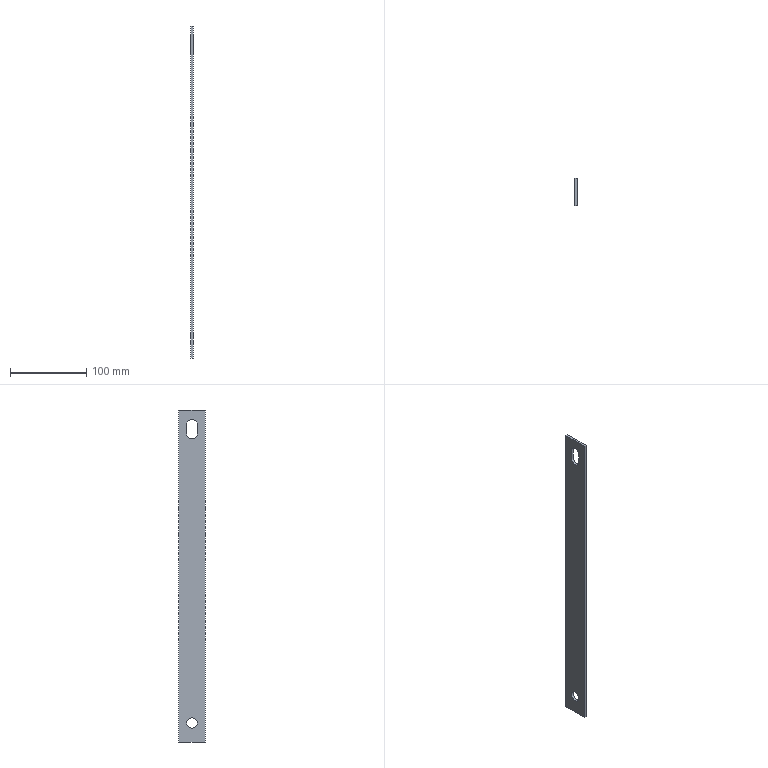Part | NX | features solid 2 | 1 solid | 11 faces | box 3 x 35 x 435 mm | volume 44310 mm3 | plane 8 | cylinder 3 | commonest cylinder face diameters 13.5 x3
STEP:
#1=CARTESIAN_POINT('',(1130.,-198.25,251.25));
#2=VERTEX_POINT('',#1);
#3=CARTESIAN_POINT('',(1130.,-211.75,251.25));
#4=VERTEX_POINT('',#3);
#5=CARTESIAN_POINT('',(1130.,-205.,251.25));
#6=DIRECTION('',(1.,0.,0.));
#7=DIRECTION('',(0.,1.,0.));
#8=AXIS2_PLACEMENT_3D('',#5,#6,#7);
#9=CIRCLE('',#8,6.75);
#10=EDGE_CURVE('',#2,#4,#9,.T.);
#11=ORIENTED_EDGE('',*,*,#10,.F.);
#12=CARTESIAN_POINT('',(1133.,-198.25,251.25));
#13=VERTEX_POINT('',#12);
#14=CARTESIAN_POINT('',(1133.,-198.25,251.25));
#15=DIRECTION('',(-1.,0.,0.));
#16=VECTOR('',#15,1000.);
#17=LINE('',#14,#16);
#18=EDGE_CURVE('',#13,#2,#17,.T.);
#19=ORIENTED_EDGE('',*,*,#18,.F.);
#20=CARTESIAN_POINT('',(1133.,-211.75,251.25));
#21=VERTEX_POINT('',#20);
#22=CARTESIAN_POINT('',(1133.,-205.,251.25));
#23=DIRECTION('',(1.,0.,0.));
#24=DIRECTION('',(0.,1.,0.));
#25=AXIS2_PLACEMENT_3D('',#22,#23,#24);
#26=CIRCLE('',#25,6.75);
#27=EDGE_CURVE('',#13,#21,#26,.T.);
#28=ORIENTED_EDGE('',*,*,#27,.T.);
#29=CARTESIAN_POINT('',(1133.,-211.75,251.25));
#30=DIRECTION('',(-1.,0.,0.));
#31=VECTOR('',#30,1000.);
#32=LINE('',#29,#31);
#33=EDGE_CURVE('',#21,#4,#32,.T.);
#34=ORIENTED_EDGE('',*,*,#33,.T.);
#35=EDGE_LOOP('',(#11,#19,#28,#34));
#36=FACE_BOUND('',#35,.T.);
#37=CARTESIAN_POINT('',(1133.,-205.,251.25));
#38=DIRECTION('',(-1.,0.,0.));
#39=DIRECTION('',(0.,1.,0.));
#40=AXIS2_PLACEMENT_3D('',#37,#38,#39);
#41=CYLINDRICAL_SURFACE('',#40,6.75);
#42=ADVANCED_FACE('',(#36),#41,.F.);
#43=CARTESIAN_POINT('',(1130.,-198.25,238.75));
#44=VERTEX_POINT('',#43);
#45=CARTESIAN_POINT('',(1130.,-198.25,251.25));
#46=DIRECTION('',(0.,0.,-1.));
#47=VECTOR('',#46,1000.);
#48=LINE('',#45,#47);
#49=EDGE_CURVE('',#2,#44,#48,.T.);
#50=ORIENTED_EDGE('',*,*,#49,.T.);
#51=CARTESIAN_POINT('',(1133.,-198.25,238.75));
#52=VERTEX_POINT('',#51);
#53=CARTESIAN_POINT('',(1133.,-198.25,238.75));
#54=DIRECTION('',(-1.,0.,0.));
#55=VECTOR('',#54,1000.);
#56=LINE('',#53,#55);
#57=EDGE_CURVE('',#52,#44,#56,.T.);
#58=ORIENTED_EDGE('',*,*,#57,.F.);
#59=CARTESIAN_POINT('',(1133.,-198.25,251.25));
#60=DIRECTION('',(0.,0.,-1.));
#61=VECTOR('',#60,1000.);
#62=LINE('',#59,#61);
#63=EDGE_CURVE('',#13,#52,#62,.T.);
#64=ORIENTED_EDGE('',*,*,#63,.F.);
#65=ORIENTED_EDGE('',*,*,#18,.T.);
#66=EDGE_LOOP('',(#50,#58,#64,#65));
#67=FACE_BOUND('',#66,.T.);
#68=CARTESIAN_POINT('',(1133.,-198.25,251.25));
#69=DIRECTION('',(0.,-1.,0.));
#70=DIRECTION('',(-1.,0.,0.));
#71=AXIS2_PLACEMENT_3D('',#68,#69,#70);
#72=PLANE('',#71);
#73=ADVANCED_FACE('',(#67),#72,.T.);
#74=CARTESIAN_POINT('',(1130.,-211.75,238.75));
#75=VERTEX_POINT('',#74);
#76=CARTESIAN_POINT('',(1130.,-205.,238.75));
#77=DIRECTION('',(1.,0.,0.));
#78=DIRECTION('',(0.,1.,0.));
#79=AXIS2_PLACEMENT_3D('',#76,#77,#78);
#80=CIRCLE('',#79,6.75);
#81=EDGE_CURVE('',#75,#44,#80,.T.);
#82=ORIENTED_EDGE('',*,*,#81,.F.);
#83=CARTESIAN_POINT('',(1133.,-211.75,238.75));
#84=VERTEX_POINT('',#83);
#85=CARTESIAN_POINT('',(1133.,-211.75,238.75));
#86=DIRECTION('',(-1.,0.,0.));
#87=VECTOR('',#86,1000.);
#88=LINE('',#85,#87);
#89=EDGE_CURVE('',#84,#75,#88,.T.);
#90=ORIENTED_EDGE('',*,*,#89,.F.);
#91=CARTESIAN_POINT('',(1133.,-205.,238.75));
#92=DIRECTION('',(1.,0.,0.));
#93=DIRECTION('',(0.,1.,0.));
#94=AXIS2_PLACEMENT_3D('',#91,#92,#93);
#95=CIRCLE('',#94,6.75);
#96=EDGE_CURVE('',#84,#52,#95,.T.);
#97=ORIENTED_EDGE('',*,*,#96,.T.);
#98=ORIENTED_EDGE('',*,*,#57,.T.);
#99=EDGE_LOOP('',(#82,#90,#97,#98));
#100=FACE_BOUND('',#99,.T.);
#101=CARTESIAN_POINT('',(1133.,-205.,238.75));
#102=DIRECTION('',(-1.,0.,0.));
#103=DIRECTION('',(0.,1.,0.));
#104=AXIS2_PLACEMENT_3D('',#101,#102,#103);
#105=CYLINDRICAL_SURFACE('',#104,6.75);
#106=ADVANCED_FACE('',(#100),#105,.F.);
#107=CARTESIAN_POINT('',(1130.,-187.5,-165.));
#108=VERTEX_POINT('',#107);
#109=CARTESIAN_POINT('',(1130.,-187.5,270.));
#110=VERTEX_POINT('',#109);
#111=CARTESIAN_POINT('',(1130.,-187.5,-30.));
#112=DIRECTION('',(0.,0.,1.));
#113=VECTOR('',#112,1000.);
#114=LINE('',#111,#113);
#115=EDGE_CURVE('',#108,#110,#114,.T.);
#116=ORIENTED_EDGE('',*,*,#115,.T.);
#117=CARTESIAN_POINT('',(1133.,-187.5,270.));
#118=VERTEX_POINT('',#117);
#119=CARTESIAN_POINT('',(1133.,-187.5,270.));
#120=DIRECTION('',(-1.,0.,0.));
#121=VECTOR('',#120,1000.);
#122=LINE('',#119,#121);
#123=EDGE_CURVE('',#118,#110,#122,.T.);
#124=ORIENTED_EDGE('',*,*,#123,.F.);
#125=CARTESIAN_POINT('',(1133.,-187.5,-165.));
#126=VERTEX_POINT('',#125);
#127=CARTESIAN_POINT('',(1133.,-187.5,-30.));
#128=DIRECTION('',(0.,0.,1.));
#129=VECTOR('',#128,1000.);
#130=LINE('',#127,#129);
#131=EDGE_CURVE('',#126,#118,#130,.T.);
#132=ORIENTED_EDGE('',*,*,#131,.F.);
#133=CARTESIAN_POINT('',(1133.,-187.5,-165.));
#134=DIRECTION('',(-1.,0.,0.));
#135=VECTOR('',#134,1000.);
#136=LINE('',#133,#135);
#137=EDGE_CURVE('',#126,#108,#136,.T.);
#138=ORIENTED_EDGE('',*,*,#137,.T.);
#139=EDGE_LOOP('',(#116,#124,#132,#138));
#140=FACE_BOUND('',#139,.T.);
#141=CARTESIAN_POINT('',(1133.,-187.5,-30.));
#142=DIRECTION('',(0.,1.,0.));
#143=DIRECTION('',(0.,0.,1.));
#144=AXIS2_PLACEMENT_3D('',#141,#142,#143);
#145=PLANE('',#144);
#146=ADVANCED_FACE('',(#140),#145,.T.);
#147=CARTESIAN_POINT('',(1130.,-222.5,270.));
#148=VERTEX_POINT('',#147);
#149=CARTESIAN_POINT('',(1130.,-187.5,270.));
#150=DIRECTION('',(0.,-1.,0.));
#151=VECTOR('',#150,1000.);
#152=LINE('',#149,#151);
#153=EDGE_CURVE('',#110,#148,#152,.T.);
#154=ORIENTED_EDGE('',*,*,#153,.T.);
#155=CARTESIAN_POINT('',(1133.,-222.5,270.));
#156=VERTEX_POINT('',#155);
#157=CARTESIAN_POINT('',(1133.,-222.5,270.));
#158=DIRECTION('',(-1.,0.,0.));
#159=VECTOR('',#158,1000.);
#160=LINE('',#157,#159);
#161=EDGE_CURVE('',#156,#148,#160,.T.);
#162=ORIENTED_EDGE('',*,*,#161,.F.);
#163=CARTESIAN_POINT('',(1133.,-187.5,270.));
#164=DIRECTION('',(0.,-1.,0.));
#165=VECTOR('',#164,1000.);
#166=LINE('',#163,#165);
#167=EDGE_CURVE('',#118,#156,#166,.T.);
#168=ORIENTED_EDGE('',*,*,#167,.F.);
#169=ORIENTED_EDGE('',*,*,#123,.T.);
#170=EDGE_LOOP('',(#154,#162,#168,#169));
#171=FACE_BOUND('',#170,.T.);
#172=CARTESIAN_POINT('',(1133.,-187.5,270.));
#173=DIRECTION('',(0.,0.,1.));
#174=DIRECTION('',(-1.,0.,0.));
#175=AXIS2_PLACEMENT_3D('',#172,#173,#174);
#176=PLANE('',#175);
#177=ADVANCED_FACE('',(#171),#176,.T.);
#178=CARTESIAN_POINT('',(1130.,-222.5,-165.));
#179=VERTEX_POINT('',#178);
#180=CARTESIAN_POINT('',(1130.,-222.5,270.));
#181=DIRECTION('',(0.,0.,-1.));
#182=VECTOR('',#181,1000.);
#183=LINE('',#180,#182);
#184=EDGE_CURVE('',#148,#179,#183,.T.);
#185=ORIENTED_EDGE('',*,*,#184,.T.);
#186=CARTESIAN_POINT('',(1133.,-222.5,-165.));
#187=VERTEX_POINT('',#186);
#188=CARTESIAN_POINT('',(1133.,-222.5,-165.));
#189=DIRECTION('',(-1.,0.,0.));
#190=VECTOR('',#189,1000.);
#191=LINE('',#188,#190);
#192=EDGE_CURVE('',#187,#179,#191,.T.);
#193=ORIENTED_EDGE('',*,*,#192,.F.);
#194=CARTESIAN_POINT('',(1133.,-222.5,270.));
#195=DIRECTION('',(0.,0.,-1.));
#196=VECTOR('',#195,1000.);
#197=LINE('',#194,#196);
#198=EDGE_CURVE('',#156,#187,#197,.T.);
#199=ORIENTED_EDGE('',*,*,#198,.F.);
#200=ORIENTED_EDGE('',*,*,#161,.T.);
#201=EDGE_LOOP('',(#185,#193,#199,#200));
#202=FACE_BOUND('',#201,.T.);
#203=CARTESIAN_POINT('',(1133.,-222.5,270.));
#204=DIRECTION('',(0.,-1.,0.));
#205=DIRECTION('',(0.,0.,-1.));
#206=AXIS2_PLACEMENT_3D('',#203,#204,#205);
#207=PLANE('',#206);
#208=ADVANCED_FACE('',(#202),#207,.T.);
#209=CARTESIAN_POINT('',(1133.,-198.25,-140.));
#210=VERTEX_POINT('',#209);
#211=CARTESIAN_POINT('',(1133.,-205.,-140.));
#212=DIRECTION('',(1.,0.,0.));
#213=DIRECTION('',(0.,1.,0.));
#214=AXIS2_PLACEMENT_3D('',#211,#212,#213);
#215=CIRCLE('',#214,6.75);
#216=EDGE_CURVE('',#210,#210,#215,.T.);
#217=ORIENTED_EDGE('',*,*,#216,.T.);
#218=EDGE_LOOP('',(#217));
#219=FACE_BOUND('',#218,.T.);
#220=CARTESIAN_POINT('',(1130.,-198.25,-140.));
#221=VERTEX_POINT('',#220);
#222=CARTESIAN_POINT('',(1130.,-205.,-140.));
#223=DIRECTION('',(1.,0.,0.));
#224=DIRECTION('',(0.,1.,0.));
#225=AXIS2_PLACEMENT_3D('',#222,#223,#224);
#226=CIRCLE('',#225,6.75);
#227=EDGE_CURVE('',#221,#221,#226,.T.);
#228=ORIENTED_EDGE('',*,*,#227,.F.);
#229=EDGE_LOOP('',(#228));
#230=FACE_BOUND('',#229,.T.);
#231=CARTESIAN_POINT('',(1133.,-205.,-140.));
#232=DIRECTION('',(-1.,0.,0.));
#233=DIRECTION('',(0.,1.,0.));
#234=AXIS2_PLACEMENT_3D('',#231,#232,#233);
#235=CYLINDRICAL_SURFACE('',#234,6.75);
#236=ADVANCED_FACE('',(#219,#230),#235,.F.);
#237=CARTESIAN_POINT('',(1130.,-222.5,-165.));
#238=DIRECTION('',(0.,1.,0.));
#239=VECTOR('',#238,1000.);
#240=LINE('',#237,#239);
#241=EDGE_CURVE('',#179,#108,#240,.T.);
#242=ORIENTED_EDGE('',*,*,#241,.T.);
#243=ORIENTED_EDGE('',*,*,#137,.F.);
#244=CARTESIAN_POINT('',(1133.,-222.5,-165.));
#245=DIRECTION('',(0.,1.,0.));
#246=VECTOR('',#245,1000.);
#247=LINE('',#244,#246);
#248=EDGE_CURVE('',#187,#126,#247,.T.);
#249=ORIENTED_EDGE('',*,*,#248,.F.);
#250=ORIENTED_EDGE('',*,*,#192,.T.);
#251=EDGE_LOOP('',(#242,#243,#249,#250));
#252=FACE_BOUND('',#251,.T.);
#253=CARTESIAN_POINT('',(1133.,-222.5,-165.));
#254=DIRECTION('',(0.,0.,-1.));
#255=DIRECTION('',(1.,0.,0.));
#256=AXIS2_PLACEMENT_3D('',#253,#254,#255);
#257=PLANE('',#256);
#258=ADVANCED_FACE('',(#252),#257,.T.);
#259=CARTESIAN_POINT('',(1130.,-211.75,238.75));
#260=DIRECTION('',(0.,0.,1.));
#261=VECTOR('',#260,1000.);
#262=LINE('',#259,#261);
#263=EDGE_CURVE('',#75,#4,#262,.T.);
#264=ORIENTED_EDGE('',*,*,#263,.T.);
#265=ORIENTED_EDGE('',*,*,#33,.F.);
#266=CARTESIAN_POINT('',(1133.,-211.75,238.75));
#267=DIRECTION('',(0.,0.,1.));
#268=VECTOR('',#267,1000.);
#269=LINE('',#266,#268);
#270=EDGE_CURVE('',#84,#21,#269,.T.);
#271=ORIENTED_EDGE('',*,*,#270,.F.);
#272=ORIENTED_EDGE('',*,*,#89,.T.);
#273=EDGE_LOOP('',(#264,#265,#271,#272));
#274=FACE_BOUND('',#273,.T.);
#275=CARTESIAN_POINT('',(1133.,-211.75,238.75));
#276=DIRECTION('',(0.,1.,0.));
#277=DIRECTION('',(1.,0.,0.));
#278=AXIS2_PLACEMENT_3D('',#275,#276,#277);
#279=PLANE('',#278);
#280=ADVANCED_FACE('',(#274),#279,.T.);
#281=ORIENTED_EDGE('',*,*,#131,.T.);
#282=ORIENTED_EDGE('',*,*,#167,.T.);
#283=ORIENTED_EDGE('',*,*,#198,.T.);
#284=ORIENTED_EDGE('',*,*,#248,.T.);
#285=EDGE_LOOP('',(#281,#282,#283,#284));
#286=FACE_BOUND('',#285,.T.);
#287=ORIENTED_EDGE('',*,*,#216,.F.);
#288=EDGE_LOOP('',(#287));
#289=FACE_BOUND('',#288,.T.);
#290=ORIENTED_EDGE('',*,*,#27,.F.);
#291=ORIENTED_EDGE('',*,*,#63,.T.);
#292=ORIENTED_EDGE('',*,*,#96,.F.);
#293=ORIENTED_EDGE('',*,*,#270,.T.);
#294=EDGE_LOOP('',(#290,#291,#292,#293));
#295=FACE_BOUND('',#294,.T.);
#296=CARTESIAN_POINT('',(1133.,-187.5,270.));
#297=DIRECTION('',(-1.,0.,0.));
#298=DIRECTION('',(0.,1.,0.));
#299=AXIS2_PLACEMENT_3D('',#296,#297,#298);
#300=PLANE('',#299);
#301=ADVANCED_FACE('',(#286,#289,#295),#300,.F.);
#302=ORIENTED_EDGE('',*,*,#115,.F.);
#303=ORIENTED_EDGE('',*,*,#241,.F.);
#304=ORIENTED_EDGE('',*,*,#184,.F.);
#305=ORIENTED_EDGE('',*,*,#153,.F.);
#306=EDGE_LOOP('',(#302,#303,#304,#305));
#307=FACE_BOUND('',#306,.T.);
#308=ORIENTED_EDGE('',*,*,#227,.T.);
#309=EDGE_LOOP('',(#308));
#310=FACE_BOUND('',#309,.T.);
#311=ORIENTED_EDGE('',*,*,#10,.T.);
#312=ORIENTED_EDGE('',*,*,#263,.F.);
#313=ORIENTED_EDGE('',*,*,#81,.T.);
#314=ORIENTED_EDGE('',*,*,#49,.F.);
#315=EDGE_LOOP('',(#311,#312,#313,#314));
#316=FACE_BOUND('',#315,.T.);
#317=CARTESIAN_POINT('',(1130.,-187.5,270.));
#318=DIRECTION('',(-1.,0.,0.));
#319=DIRECTION('',(0.,1.,0.));
#320=AXIS2_PLACEMENT_3D('',#317,#318,#319);
#321=PLANE('',#320);
#322=ADVANCED_FACE('',(#307,#310,#316),#321,.T.);
#323=CLOSED_SHELL('',(#42,#73,#106,#146,#177,#208,#236,#258,#280,#301,#322));
#324=MANIFOLD_SOLID_BREP('',#323);
#325=(LENGTH_UNIT()NAMED_UNIT(*)SI_UNIT(.MILLI.,.METRE.));
#326=UNCERTAINTY_MEASURE_WITH_UNIT(LENGTH_MEASURE(0.00001),#325,'','');
#327=(NAMED_UNIT(*)PLANE_ANGLE_UNIT()SI_UNIT($,.RADIAN.));
#328=(NAMED_UNIT(*)SI_UNIT($,.STERADIAN.)SOLID_ANGLE_UNIT());
#329=(GEOMETRIC_REPRESENTATION_CONTEXT(3)GLOBAL_UNCERTAINTY_ASSIGNED_CONTEXT((#326))GLOBAL_UNIT_ASSIGNED_CONTEXT((#325,#327,#328))REPRESENTATION_CONTEXT('',''));
#330=ADVANCED_BREP_SHAPE_REPRESENTATION('',(#324),#329);